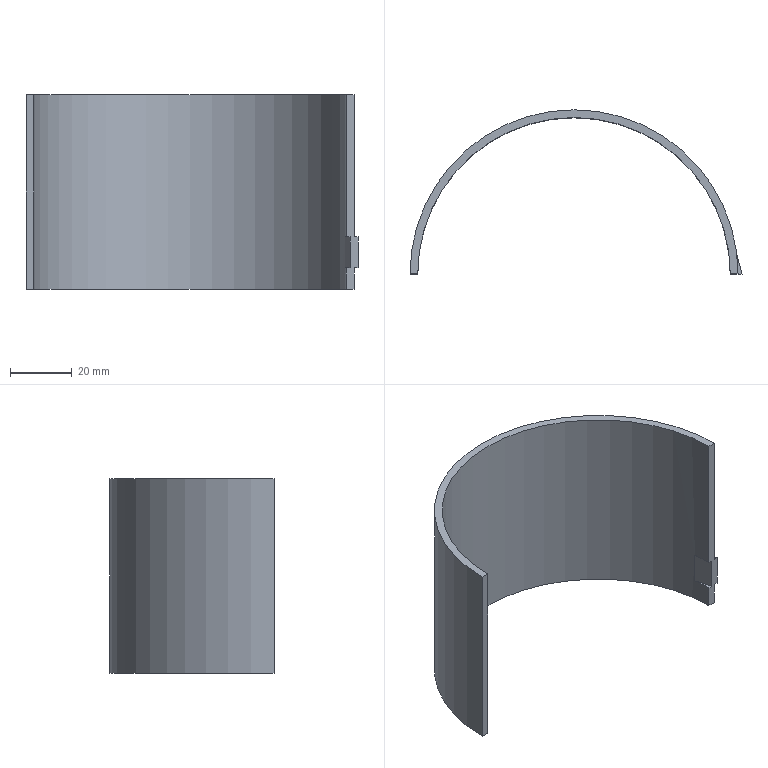Part | NX | features DATUM_CSYS 8, SKETCH 6, EXTRUDE 4, DATUM_PLANE 1, UNITE 1 | 1 solid | 13 faces | box 107.287 x 53 x 63 mm | volume 25608 mm3 | plane 11 | cylinder 2 | commonest cylinder face diameters 101 x1 106 x1
STEP:
#1=CARTESIAN_POINT('',(53.,0.,3.));
#2=VERTEX_POINT('',#1);
#3=CARTESIAN_POINT('',(50.5,0.,3.));
#4=VERTEX_POINT('',#3);
#5=CARTESIAN_POINT('',(52.691,0.,3.));
#6=DIRECTION('',(-1.,0.,0.));
#7=VECTOR('',#6,1000.);
#8=LINE('',#5,#7);
#9=EDGE_CURVE('',#2,#4,#8,.T.);
#10=ORIENTED_EDGE('',*,*,#9,.F.);
#11=CARTESIAN_POINT('',(53.,0.,10.));
#12=VERTEX_POINT('',#11);
#13=CARTESIAN_POINT('',(53.,0.,66.));
#14=DIRECTION('',(0.,0.,-1.));
#15=VECTOR('',#14,1000.);
#16=LINE('',#13,#15);
#17=EDGE_CURVE('',#12,#2,#16,.T.);
#18=ORIENTED_EDGE('',*,*,#17,.F.);
#19=CARTESIAN_POINT('',(54.287,0.,10.));
#20=VERTEX_POINT('',#19);
#21=CARTESIAN_POINT('',(52.691,0.,10.));
#22=DIRECTION('',(1.,0.,0.));
#23=VECTOR('',#22,1000.);
#24=LINE('',#21,#23);
#25=EDGE_CURVE('',#12,#20,#24,.T.);
#26=ORIENTED_EDGE('',*,*,#25,.T.);
#27=CARTESIAN_POINT('',(54.287,0.,20.));
#28=VERTEX_POINT('',#27);
#29=CARTESIAN_POINT('',(54.287,0.,20.));
#30=DIRECTION('',(0.,0.,-1.));
#31=VECTOR('',#30,1000.);
#32=LINE('',#29,#31);
#33=EDGE_CURVE('',#28,#20,#32,.T.);
#34=ORIENTED_EDGE('',*,*,#33,.F.);
#35=CARTESIAN_POINT('',(53.,0.,20.));
#36=VERTEX_POINT('',#35);
#37=CARTESIAN_POINT('',(52.691,0.,20.));
#38=DIRECTION('',(1.,0.,0.));
#39=VECTOR('',#38,1000.);
#40=LINE('',#37,#39);
#41=EDGE_CURVE('',#36,#28,#40,.T.);
#42=ORIENTED_EDGE('',*,*,#41,.F.);
#43=CARTESIAN_POINT('',(53.,0.,66.));
#44=VERTEX_POINT('',#43);
#45=CARTESIAN_POINT('',(53.,0.,66.));
#46=DIRECTION('',(0.,0.,-1.));
#47=VECTOR('',#46,1000.);
#48=LINE('',#45,#47);
#49=EDGE_CURVE('',#44,#36,#48,.T.);
#50=ORIENTED_EDGE('',*,*,#49,.F.);
#51=CARTESIAN_POINT('',(50.5,0.,66.));
#52=VERTEX_POINT('',#51);
#53=CARTESIAN_POINT('',(50.5,0.,66.));
#54=DIRECTION('',(1.,0.,0.));
#55=VECTOR('',#54,1000.);
#56=LINE('',#53,#55);
#57=EDGE_CURVE('',#52,#44,#56,.T.);
#58=ORIENTED_EDGE('',*,*,#57,.F.);
#59=CARTESIAN_POINT('',(50.5,0.,20.));
#60=VERTEX_POINT('',#59);
#61=CARTESIAN_POINT('',(50.5,0.,66.));
#62=DIRECTION('',(0.,0.,-1.));
#63=VECTOR('',#62,1000.);
#64=LINE('',#61,#63);
#65=EDGE_CURVE('',#52,#60,#64,.T.);
#66=ORIENTED_EDGE('',*,*,#65,.T.);
#67=CARTESIAN_POINT('',(51.75,0.,20.));
#68=VERTEX_POINT('',#67);
#69=CARTESIAN_POINT('',(50.5,0.,20.));
#70=DIRECTION('',(1.,0.,0.));
#71=VECTOR('',#70,1000.);
#72=LINE('',#69,#71);
#73=EDGE_CURVE('',#60,#68,#72,.T.);
#74=ORIENTED_EDGE('',*,*,#73,.T.);
#75=CARTESIAN_POINT('',(51.75,0.,10.));
#76=VERTEX_POINT('',#75);
#77=CARTESIAN_POINT('',(51.75,0.,20.));
#78=DIRECTION('',(0.,0.,-1.));
#79=VECTOR('',#78,1000.);
#80=LINE('',#77,#79);
#81=EDGE_CURVE('',#68,#76,#80,.T.);
#82=ORIENTED_EDGE('',*,*,#81,.T.);
#83=CARTESIAN_POINT('',(50.5,0.,10.));
#84=VERTEX_POINT('',#83);
#85=CARTESIAN_POINT('',(50.5,0.,10.));
#86=DIRECTION('',(1.,0.,0.));
#87=VECTOR('',#86,1000.);
#88=LINE('',#85,#87);
#89=EDGE_CURVE('',#84,#76,#88,.T.);
#90=ORIENTED_EDGE('',*,*,#89,.F.);
#91=CARTESIAN_POINT('',(50.5,0.,66.));
#92=DIRECTION('',(0.,0.,-1.));
#93=VECTOR('',#92,1000.);
#94=LINE('',#91,#93);
#95=EDGE_CURVE('',#84,#4,#94,.T.);
#96=ORIENTED_EDGE('',*,*,#95,.T.);
#97=EDGE_LOOP('',(#10,#18,#26,#34,#42,#50,#58,#66,#74,#82,#90,#96));
#98=FACE_BOUND('',#97,.T.);
#99=CARTESIAN_POINT('',(52.691,0.,20.));
#100=DIRECTION('',(0.,1.,0.));
#101=DIRECTION('',(0.,0.,1.));
#102=AXIS2_PLACEMENT_3D('',#99,#100,#101);
#103=PLANE('',#102);
#104=ADVANCED_FACE('',(#98),#103,.F.);
#105=CARTESIAN_POINT('',(-53.,0.,3.));
#106=VERTEX_POINT('',#105);
#107=CARTESIAN_POINT('',(0.,0.,3.));
#108=DIRECTION('',(0.,0.,-1.));
#109=DIRECTION('',(1.,0.,0.));
#110=AXIS2_PLACEMENT_3D('',#107,#108,#109);
#111=CIRCLE('',#110,53.);
#112=EDGE_CURVE('',#106,#2,#111,.T.);
#113=ORIENTED_EDGE('',*,*,#112,.F.);
#114=CARTESIAN_POINT('',(-53.,0.,66.));
#115=VERTEX_POINT('',#114);
#116=CARTESIAN_POINT('',(-53.,0.,66.));
#117=DIRECTION('',(0.,0.,-1.));
#118=VECTOR('',#117,1000.);
#119=LINE('',#116,#118);
#120=EDGE_CURVE('',#115,#106,#119,.T.);
#121=ORIENTED_EDGE('',*,*,#120,.F.);
#122=CARTESIAN_POINT('',(0.,0.,66.));
#123=DIRECTION('',(0.,0.,1.));
#124=DIRECTION('',(1.,0.,0.));
#125=AXIS2_PLACEMENT_3D('',#122,#123,#124);
#126=CIRCLE('',#125,53.);
#127=EDGE_CURVE('',#44,#115,#126,.T.);
#128=ORIENTED_EDGE('',*,*,#127,.F.);
#129=ORIENTED_EDGE('',*,*,#49,.T.);
#130=CARTESIAN_POINT('',(52.691,5.718,20.));
#131=VERTEX_POINT('',#130);
#132=CARTESIAN_POINT('',(0.,0.,20.));
#133=DIRECTION('',(0.,0.,-1.));
#134=DIRECTION('',(-1.,0.,0.));
#135=AXIS2_PLACEMENT_3D('',#132,#133,#134);
#136=CIRCLE('',#135,53.);
#137=EDGE_CURVE('',#36,#131,#136,.F.);
#138=ORIENTED_EDGE('',*,*,#137,.T.);
#139=CARTESIAN_POINT('',(52.691,5.718,10.));
#140=VERTEX_POINT('',#139);
#141=CARTESIAN_POINT('',(52.691,5.718,66.));
#142=DIRECTION('',(0.,0.,-1.));
#143=VECTOR('',#142,1000.);
#144=LINE('',#141,#143);
#145=EDGE_CURVE('',#131,#140,#144,.T.);
#146=ORIENTED_EDGE('',*,*,#145,.T.);
#147=CARTESIAN_POINT('',(0.,0.,10.));
#148=DIRECTION('',(0.,0.,-1.));
#149=DIRECTION('',(-1.,0.,0.));
#150=AXIS2_PLACEMENT_3D('',#147,#148,#149);
#151=CIRCLE('',#150,53.);
#152=EDGE_CURVE('',#12,#140,#151,.F.);
#153=ORIENTED_EDGE('',*,*,#152,.F.);
#154=ORIENTED_EDGE('',*,*,#17,.T.);
#155=EDGE_LOOP('',(#113,#121,#128,#129,#138,#146,#153,#154));
#156=FACE_BOUND('',#155,.T.);
#157=CARTESIAN_POINT('',(0.,0.,66.));
#158=DIRECTION('',(0.,0.,-1.));
#159=DIRECTION('',(-1.,0.,0.));
#160=AXIS2_PLACEMENT_3D('',#157,#158,#159);
#161=CYLINDRICAL_SURFACE('',#160,53.);
#162=ADVANCED_FACE('',(#156),#161,.T.);
#163=CARTESIAN_POINT('',(-50.5,0.,3.));
#164=VERTEX_POINT('',#163);
#165=CARTESIAN_POINT('',(0.,0.,3.));
#166=DIRECTION('',(0.,0.,-1.));
#167=DIRECTION('',(1.,0.,0.));
#168=AXIS2_PLACEMENT_3D('',#165,#166,#167);
#169=CIRCLE('',#168,50.5);
#170=EDGE_CURVE('',#164,#4,#169,.T.);
#171=ORIENTED_EDGE('',*,*,#170,.T.);
#172=ORIENTED_EDGE('',*,*,#95,.F.);
#173=CARTESIAN_POINT('',(50.136,6.048,10.));
#174=VERTEX_POINT('',#173);
#175=CARTESIAN_POINT('',(0.,0.,10.));
#176=DIRECTION('',(0.,0.,-1.));
#177=DIRECTION('',(1.,0.,0.));
#178=AXIS2_PLACEMENT_3D('',#175,#176,#177);
#179=CIRCLE('',#178,50.5);
#180=EDGE_CURVE('',#174,#84,#179,.T.);
#181=ORIENTED_EDGE('',*,*,#180,.F.);
#182=CARTESIAN_POINT('',(50.136,6.048,20.));
#183=VERTEX_POINT('',#182);
#184=CARTESIAN_POINT('',(50.136,6.048,20.));
#185=DIRECTION('',(0.,0.,-1.));
#186=VECTOR('',#185,1000.);
#187=LINE('',#184,#186);
#188=EDGE_CURVE('',#183,#174,#187,.T.);
#189=ORIENTED_EDGE('',*,*,#188,.F.);
#190=CARTESIAN_POINT('',(0.,0.,20.));
#191=DIRECTION('',(0.,0.,-1.));
#192=DIRECTION('',(1.,0.,0.));
#193=AXIS2_PLACEMENT_3D('',#190,#191,#192);
#194=CIRCLE('',#193,50.5);
#195=EDGE_CURVE('',#183,#60,#194,.T.);
#196=ORIENTED_EDGE('',*,*,#195,.T.);
#197=ORIENTED_EDGE('',*,*,#65,.F.);
#198=CARTESIAN_POINT('',(-50.5,0.,66.));
#199=VERTEX_POINT('',#198);
#200=CARTESIAN_POINT('',(0.,0.,66.));
#201=DIRECTION('',(0.,0.,-1.));
#202=DIRECTION('',(1.,0.,0.));
#203=AXIS2_PLACEMENT_3D('',#200,#201,#202);
#204=CIRCLE('',#203,50.5);
#205=EDGE_CURVE('',#199,#52,#204,.T.);
#206=ORIENTED_EDGE('',*,*,#205,.F.);
#207=CARTESIAN_POINT('',(-50.5,0.,66.));
#208=DIRECTION('',(0.,0.,-1.));
#209=VECTOR('',#208,1000.);
#210=LINE('',#207,#209);
#211=EDGE_CURVE('',#199,#164,#210,.T.);
#212=ORIENTED_EDGE('',*,*,#211,.T.);
#213=EDGE_LOOP('',(#171,#172,#181,#189,#196,#197,#206,#212));
#214=FACE_BOUND('',#213,.T.);
#215=CARTESIAN_POINT('',(0.,0.,66.));
#216=DIRECTION('',(0.,0.,-1.));
#217=DIRECTION('',(-1.,0.,0.));
#218=AXIS2_PLACEMENT_3D('',#215,#216,#217);
#219=CYLINDRICAL_SURFACE('',#218,50.5);
#220=ADVANCED_FACE('',(#214),#219,.F.);
#221=CARTESIAN_POINT('',(-53.,0.,3.));
#222=DIRECTION('',(-1.,0.,0.));
#223=VECTOR('',#222,1000.);
#224=LINE('',#221,#223);
#225=EDGE_CURVE('',#164,#106,#224,.T.);
#226=ORIENTED_EDGE('',*,*,#225,.F.);
#227=ORIENTED_EDGE('',*,*,#211,.F.);
#228=CARTESIAN_POINT('',(-53.,0.,66.));
#229=DIRECTION('',(1.,0.,0.));
#230=VECTOR('',#229,1000.);
#231=LINE('',#228,#230);
#232=EDGE_CURVE('',#115,#199,#231,.T.);
#233=ORIENTED_EDGE('',*,*,#232,.F.);
#234=ORIENTED_EDGE('',*,*,#120,.T.);
#235=EDGE_LOOP('',(#226,#227,#233,#234));
#236=FACE_BOUND('',#235,.T.);
#237=CARTESIAN_POINT('',(-53.,0.,66.));
#238=DIRECTION('',(0.,1.,0.));
#239=DIRECTION('',(0.,0.,1.));
#240=AXIS2_PLACEMENT_3D('',#237,#238,#239);
#241=PLANE('',#240);
#242=ADVANCED_FACE('',(#236),#241,.F.);
#243=ORIENTED_EDGE('',*,*,#145,.F.);
#244=CARTESIAN_POINT('',(52.691,6.048,20.));
#245=VERTEX_POINT('',#244);
#246=CARTESIAN_POINT('',(52.691,6.048,20.));
#247=DIRECTION('',(0.,-1.,0.));
#248=VECTOR('',#247,1000.);
#249=LINE('',#246,#248);
#250=EDGE_CURVE('',#245,#131,#249,.T.);
#251=ORIENTED_EDGE('',*,*,#250,.F.);
#252=CARTESIAN_POINT('',(52.691,6.048,10.));
#253=VERTEX_POINT('',#252);
#254=CARTESIAN_POINT('',(52.691,6.048,20.));
#255=DIRECTION('',(0.,0.,-1.));
#256=VECTOR('',#255,1000.);
#257=LINE('',#254,#256);
#258=EDGE_CURVE('',#245,#253,#257,.T.);
#259=ORIENTED_EDGE('',*,*,#258,.T.);
#260=CARTESIAN_POINT('',(52.691,6.048,10.));
#261=DIRECTION('',(0.,-1.,0.));
#262=VECTOR('',#261,1000.);
#263=LINE('',#260,#262);
#264=EDGE_CURVE('',#253,#140,#263,.T.);
#265=ORIENTED_EDGE('',*,*,#264,.T.);
#266=EDGE_LOOP('',(#243,#251,#259,#265));
#267=FACE_BOUND('',#266,.T.);
#268=CARTESIAN_POINT('',(52.691,6.048,20.));
#269=DIRECTION('',(1.,0.,0.));
#270=DIRECTION('',(0.,1.,0.));
#271=AXIS2_PLACEMENT_3D('',#268,#269,#270);
#272=PLANE('',#271);
#273=ADVANCED_FACE('',(#267),#272,.F.);
#274=ORIENTED_EDGE('',*,*,#137,.F.);
#275=ORIENTED_EDGE('',*,*,#41,.T.);
#276=CARTESIAN_POINT('',(54.287,0.,20.));
#277=DIRECTION('',(-0.2551,0.9669,0.));
#278=VECTOR('',#277,1000.);
#279=LINE('',#276,#278);
#280=EDGE_CURVE('',#28,#245,#279,.T.);
#281=ORIENTED_EDGE('',*,*,#280,.T.);
#282=ORIENTED_EDGE('',*,*,#250,.T.);
#283=EDGE_LOOP('',(#274,#275,#281,#282));
#284=FACE_BOUND('',#283,.T.);
#285=CARTESIAN_POINT('',(0.,0.,20.));
#286=DIRECTION('',(0.,0.,-1.));
#287=DIRECTION('',(-1.,0.,0.));
#288=AXIS2_PLACEMENT_3D('',#285,#286,#287);
#289=PLANE('',#288);
#290=ADVANCED_FACE('',(#284),#289,.F.);
#291=ORIENTED_EDGE('',*,*,#25,.F.);
#292=ORIENTED_EDGE('',*,*,#152,.T.);
#293=ORIENTED_EDGE('',*,*,#264,.F.);
#294=CARTESIAN_POINT('',(54.287,0.,10.));
#295=DIRECTION('',(-0.2551,0.9669,0.));
#296=VECTOR('',#295,1000.);
#297=LINE('',#294,#296);
#298=EDGE_CURVE('',#20,#253,#297,.T.);
#299=ORIENTED_EDGE('',*,*,#298,.F.);
#300=EDGE_LOOP('',(#291,#292,#293,#299));
#301=FACE_BOUND('',#300,.T.);
#302=CARTESIAN_POINT('',(0.,0.,10.));
#303=DIRECTION('',(0.,0.,-1.));
#304=DIRECTION('',(-1.,0.,0.));
#305=AXIS2_PLACEMENT_3D('',#302,#303,#304);
#306=PLANE('',#305);
#307=ADVANCED_FACE('',(#301),#306,.T.);
#308=ORIENTED_EDGE('',*,*,#298,.T.);
#309=ORIENTED_EDGE('',*,*,#258,.F.);
#310=ORIENTED_EDGE('',*,*,#280,.F.);
#311=ORIENTED_EDGE('',*,*,#33,.T.);
#312=EDGE_LOOP('',(#308,#309,#310,#311));
#313=FACE_BOUND('',#312,.T.);
#314=CARTESIAN_POINT('',(54.287,0.,20.));
#315=DIRECTION('',(-0.9669,-0.2551,0.));
#316=DIRECTION('',(0.2551,-0.9669,0.));
#317=AXIS2_PLACEMENT_3D('',#314,#315,#316);
#318=PLANE('',#317);
#319=ADVANCED_FACE('',(#313),#318,.F.);
#320=ORIENTED_EDGE('',*,*,#232,.T.);
#321=ORIENTED_EDGE('',*,*,#205,.T.);
#322=ORIENTED_EDGE('',*,*,#57,.T.);
#323=ORIENTED_EDGE('',*,*,#127,.T.);
#324=EDGE_LOOP('',(#320,#321,#322,#323));
#325=FACE_BOUND('',#324,.T.);
#326=CARTESIAN_POINT('',(0.,0.,66.));
#327=DIRECTION('',(0.,0.,-1.));
#328=DIRECTION('',(-1.,0.,0.));
#329=AXIS2_PLACEMENT_3D('',#326,#327,#328);
#330=PLANE('',#329);
#331=ADVANCED_FACE('',(#325),#330,.F.);
#332=CARTESIAN_POINT('',(51.75,0.,10.));
#333=DIRECTION('',(-0.2578,0.9662,0.));
#334=VECTOR('',#333,1000.);
#335=LINE('',#332,#334);
#336=EDGE_CURVE('',#174,#76,#335,.F.);
#337=ORIENTED_EDGE('',*,*,#336,.T.);
#338=ORIENTED_EDGE('',*,*,#81,.F.);
#339=CARTESIAN_POINT('',(51.75,0.,20.));
#340=DIRECTION('',(-0.2578,0.9662,0.));
#341=VECTOR('',#340,1000.);
#342=LINE('',#339,#341);
#343=EDGE_CURVE('',#183,#68,#342,.F.);
#344=ORIENTED_EDGE('',*,*,#343,.F.);
#345=ORIENTED_EDGE('',*,*,#188,.T.);
#346=EDGE_LOOP('',(#337,#338,#344,#345));
#347=FACE_BOUND('',#346,.T.);
#348=CARTESIAN_POINT('',(51.75,0.,20.));
#349=DIRECTION('',(-0.9662,-0.2578,0.));
#350=DIRECTION('',(0.2578,-0.9662,0.));
#351=AXIS2_PLACEMENT_3D('',#348,#349,#350);
#352=PLANE('',#351);
#353=ADVANCED_FACE('',(#347),#352,.T.);
#354=ORIENTED_EDGE('',*,*,#195,.F.);
#355=ORIENTED_EDGE('',*,*,#343,.T.);
#356=ORIENTED_EDGE('',*,*,#73,.F.);
#357=EDGE_LOOP('',(#354,#355,#356));
#358=FACE_BOUND('',#357,.T.);
#359=CARTESIAN_POINT('',(0.,0.,20.));
#360=DIRECTION('',(0.,0.,-1.));
#361=DIRECTION('',(-1.,0.,0.));
#362=AXIS2_PLACEMENT_3D('',#359,#360,#361);
#363=PLANE('',#362);
#364=ADVANCED_FACE('',(#358),#363,.T.);
#365=ORIENTED_EDGE('',*,*,#180,.T.);
#366=ORIENTED_EDGE('',*,*,#89,.T.);
#367=ORIENTED_EDGE('',*,*,#336,.F.);
#368=EDGE_LOOP('',(#365,#366,#367));
#369=FACE_BOUND('',#368,.T.);
#370=CARTESIAN_POINT('',(0.,0.,10.));
#371=DIRECTION('',(0.,0.,-1.));
#372=DIRECTION('',(-1.,0.,0.));
#373=AXIS2_PLACEMENT_3D('',#370,#371,#372);
#374=PLANE('',#373);
#375=ADVANCED_FACE('',(#369),#374,.F.);
#376=ORIENTED_EDGE('',*,*,#9,.T.);
#377=ORIENTED_EDGE('',*,*,#170,.F.);
#378=ORIENTED_EDGE('',*,*,#225,.T.);
#379=ORIENTED_EDGE('',*,*,#112,.T.);
#380=EDGE_LOOP('',(#376,#377,#378,#379));
#381=FACE_BOUND('',#380,.T.);
#382=CARTESIAN_POINT('',(0.,0.,3.));
#383=DIRECTION('',(0.,0.,-1.));
#384=DIRECTION('',(-1.,0.,0.));
#385=AXIS2_PLACEMENT_3D('',#382,#383,#384);
#386=PLANE('',#385);
#387=ADVANCED_FACE('',(#381),#386,.T.);
#388=CLOSED_SHELL('',(#104,#162,#220,#242,#273,#290,#307,#319,#331,#353,#364,#375,#387));
#389=MANIFOLD_SOLID_BREP('',#388);
#390=(LENGTH_UNIT()NAMED_UNIT(*)SI_UNIT(.MILLI.,.METRE.));
#391=UNCERTAINTY_MEASURE_WITH_UNIT(LENGTH_MEASURE(0.00001),#390,'','');
#392=(NAMED_UNIT(*)PLANE_ANGLE_UNIT()SI_UNIT($,.RADIAN.));
#393=(NAMED_UNIT(*)SI_UNIT($,.STERADIAN.)SOLID_ANGLE_UNIT());
#394=(GEOMETRIC_REPRESENTATION_CONTEXT(3)GLOBAL_UNCERTAINTY_ASSIGNED_CONTEXT((#391))GLOBAL_UNIT_ASSIGNED_CONTEXT((#390,#392,#393))REPRESENTATION_CONTEXT('',''));
#395=ADVANCED_BREP_SHAPE_REPRESENTATION('',(#389),#394);